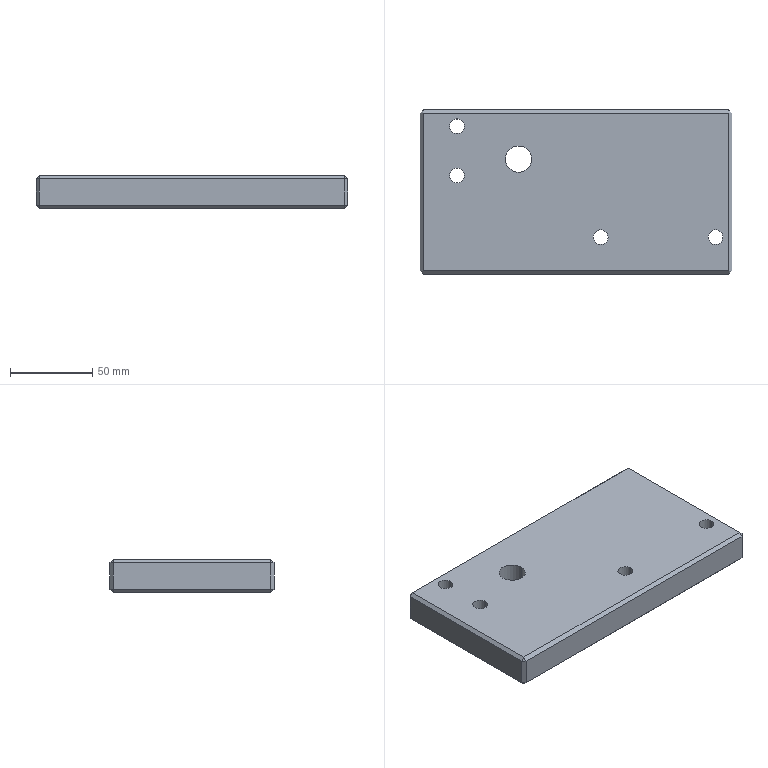Part | STEP file | Foot seat plate 2 | 1 solid | 36 faces | box 190 x 100 x 20 mm | volume 368452 mm3 | plane 26 | cylinder 10 | commonest cylinder face diameters 9 x8 16 x2